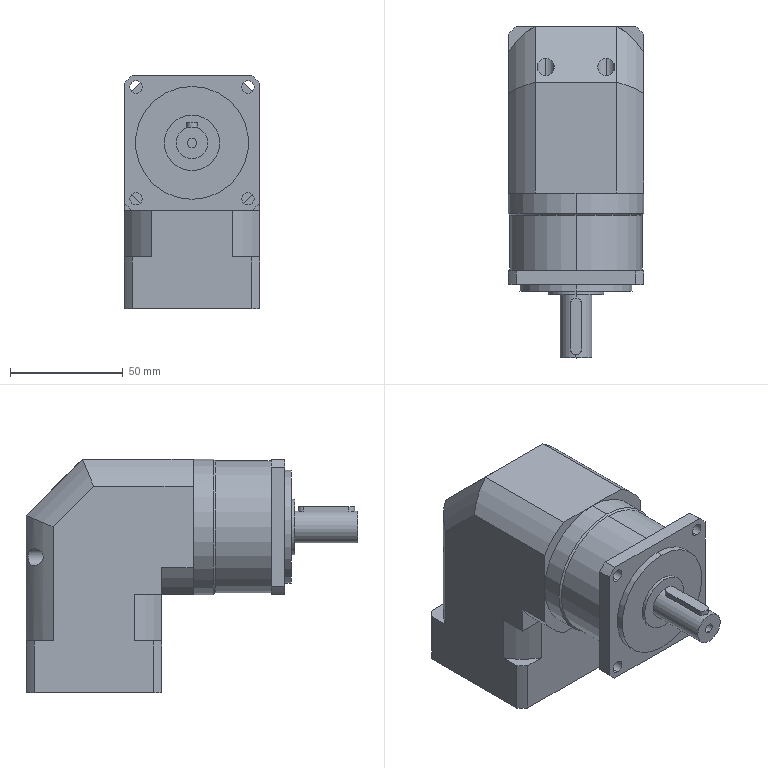Part | SolidWorks | features BaseBody 1 | 1 solid | 168 faces | box 60 x 147 x 103.5 mm | volume 479468 mm3 | cylinder 89 | plane 53 | cone 26 | commonest cylinder face diameters 3.3 x24 70 x10 4.5 x8 5.5 x8 7.5 x8 80 x8